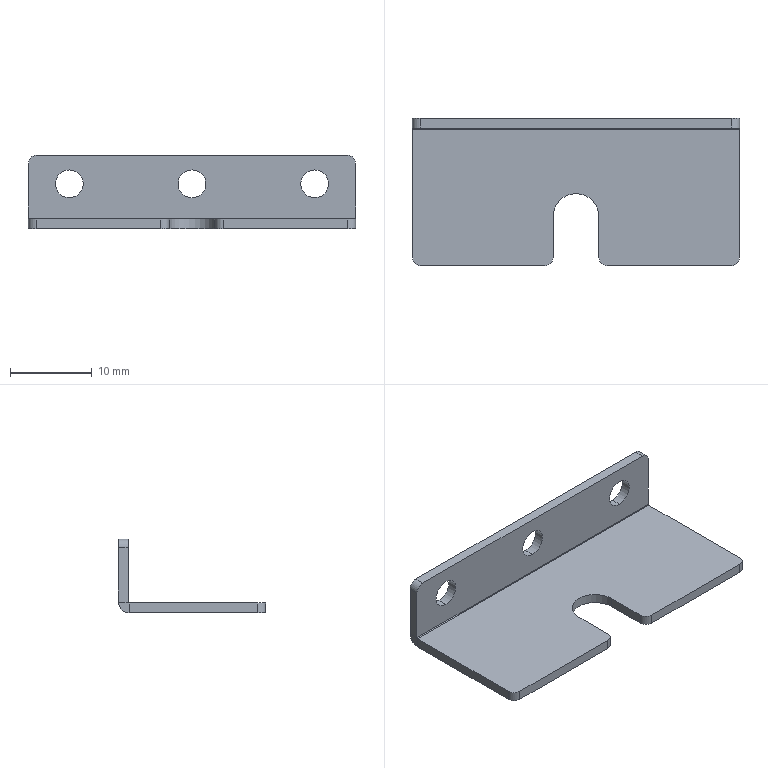Part | STEP file | side push connection plate | 1 solid | 30 faces | box 40 x 18 x 9 mm | volume 1135 mm3 | cylinder 15 | plane 15 | commonest cylinder face diameters 2 x6 3.4 x6 0.2 x1 2.6 x1 5.6 x1